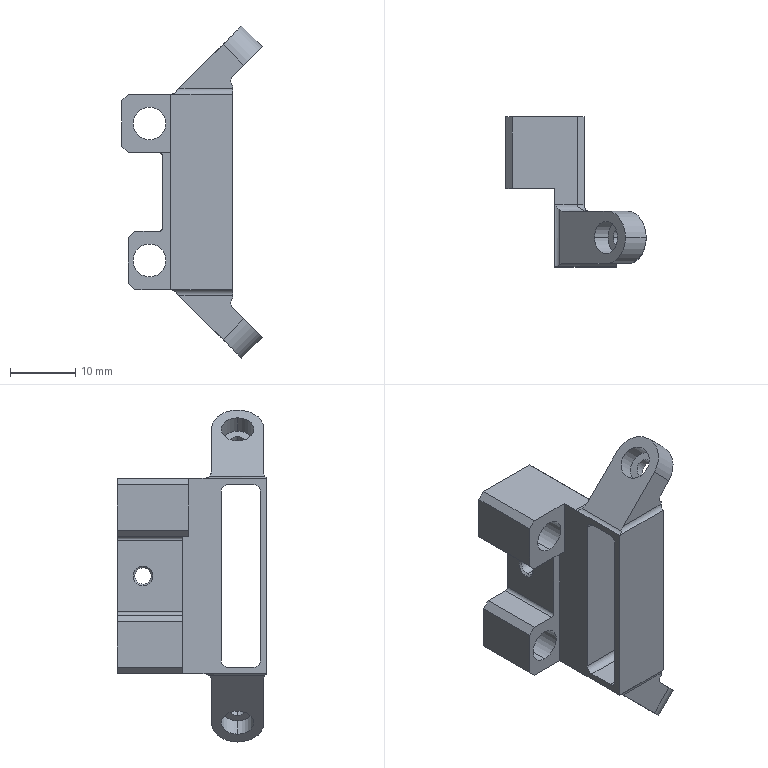NC program | NX | posted with a generic post | part box 21.534 x 23 x 50.912 mm
Lines 6134 to 6474 of 6474:
(PLANAR_MILL_1 , TOOL : D6R1)
N12248 T02 M6
N12250 G54
N12252 G17 G0 G90 X-0.5 Y-15.853 B0. C0. S1061 M3
N12254 G43 Z50. H2
N12256 Z-12.5
N12258 G94 G1 Z-14.5 F250.
N12260 X0.293 Y-13.646
N12262 X-0.414 Y-14.353
N12264 X-1.414 Y-15.353
N12266 G2 X-7. Y-17.667 R7.9
N12268 G1 X-14.
N12270 G2 X-19.586 Y-15.353 R7.9
N12272 G1 X-20.586 Y-14.353
N12274 G2 X-22.9 Y-8.767 R7.9
N12276 G1 Y0.233
N12278 G2 X-20.586 Y5.819 R7.9
N12280 G1 X-19.586 Y6.819
N12282 G2 X-14. Y9.133 R7.9
N12284 G1 X14.
N12286 G2 X19.586 Y6.819 R7.9
N12288 G1 X20.586 Y5.819
N12290 G2 X22.9 Y0.233 R7.9
N12292 G1 Y-9.767
N12294 G2 X20.586 Y-15.353 R7.9
N12296 G1 X19.586 Y-16.353
N12298 G2 X14. Y-18.667 R7.9
N12300 G1 X7.
N12302 G2 X1.414 Y-16.353 R7.9
N12304 G1 X0.414 Y-15.353
N12306 X-0.293 Y-14.646
N12308 X-0.5 Y-15.853
N12310 Z-12.5
N12312 G0 Z50.
N12314 X0.5 Y-9.61
N12316 Z-12.5
N12318 G1 Z-14.5
N12320 X-1.404 Y-11.949
N12322 X-2.111 Y-12.656
N12324 X-3.111 Y-13.656
N12326 G2 X-7. Y-15.267 R5.5
N12328 G1 X-14.
N12330 G2 X-17.889 Y-13.656 R5.5
N12332 G1 X-18.889 Y-12.656
N12334 G2 X-20.5 Y-8.767 R5.5
N12336 G1 Y0.233
N12338 G2 X-18.889 Y4.122 R5.5
N12340 G1 X-17.889 Y5.122
N12342 G2 X-14. Y6.733 R5.5
N12344 G1 X14.
N12346 G2 X17.889 Y5.122 R5.5
N12348 G1 X18.889 Y4.122
N12350 G2 X20.5 Y0.233 R5.5
N12352 G1 Y-9.767
N12354 G2 X18.889 Y-13.656 R5.5
N12356 G1 X17.889 Y-14.656
N12358 G2 X14. Y-16.267 R5.5
N12360 G1 X7.
N12362 G2 X3.111 Y-14.656 R5.5
N12364 G1 X2.111 Y-13.656
N12366 X1.404 Y-12.949
N12368 X0.5 Y-9.61
N12370 Z-12.5
N12372 G0 Z50.
N12374 X-0.98 Y-8.13
N12376 Z-12.5
N12378 G1 Z-14.5
N12380 X-3.808 Y-10.959
N12382 X-4.808 Y-11.959
N12384 G2 X-7. Y-12.867 R3.1
N12386 G1 X-14.
N12388 G2 X-16.192 Y-11.959 R3.1
N12390 G1 X-17.192 Y-10.959
N12392 G2 X-18.1 Y-8.767 R3.1
N12394 G1 Y0.233
N12396 G2 X-17.192 Y2.425 R3.1
N12398 G1 X-16.192 Y3.425
N12400 G2 X-14. Y4.333 R3.1
N12402 G1 X14.
N12404 G2 X16.192 Y3.425 R3.1
N12406 G1 X17.192 Y2.425
N12408 G2 X18.1 Y0.233 R3.1
N12410 G1 Y-9.767
N12412 G2 X17.192 Y-11.959 R3.1
N12414 G1 X16.192 Y-12.959
N12416 G2 X14. Y-13.867 R3.1
N12418 G1 X7.
N12420 G2 X4.808 Y-12.959 R3.1
N12422 G1 X3.808 Y-11.959
N12424 X0.98 Y-9.13
N12426 Z-12.5
N12428 G0 Z50.
(PLANAR_MILL_1_COPY , TOOL : D6R1)
N12430 X-1.05 Y-8.06
N12432 Z-12.5
N12434 G1 Z-14.5
N12436 X-3.879 Y-10.888
N12438 X-4.879 Y-11.888
N12440 G2 X-7. Y-12.767 R3.
N12442 G1 X-14.
N12444 G2 X-16.121 Y-11.888 R3.
N12446 G1 X-17.121 Y-10.888
N12448 G2 X-18. Y-8.767 R3.
N12450 G1 Y0.233
N12452 G2 X-17.121 Y2.354 R3.
N12454 G1 X-16.121 Y3.354
N12456 G2 X-14. Y4.233 R3.
N12458 G1 X14.
N12460 G2 X16.121 Y3.354 R3.
N12462 G1 X17.121 Y2.354
N12464 G2 X18. Y0.233 R3.
N12466 G1 Y-9.767
N12468 G2 X17.121 Y-11.888 R3.
N12470 G1 X16.121 Y-12.888
N12472 G2 X14. Y-13.767 R3.
N12474 G1 X7.
N12476 G2 X4.879 Y-12.888 R3.
N12478 G1 X3.879 Y-11.888
N12480 X1.05 Y-9.06
N12482 Z-12.5
N12484 G0 Z50.
(FLOOR_FACING_1_COPY , TOOL : D6R1)
N12486 G19 G43 Y62.5 Z-8.5 B-180. C0. H2
N12488 X0.
N12490 Y9.233
N12492 G1 Y6.233
N12494 Z-18.8
N12496 X-12.04
N12498 Z-18.7
N12500 X12.04
N12502 Z-18.8
N12504 X0.
N12506 Z-21.5
N12508 X-14.134
N12510 X-14.423 Z-21.
N12512 X-14.74
N12514 Z-16.
N12516 X14.74
N12518 Z-21.
N12520 X14.423
N12522 X14.134 Z-21.5
N12524 X0.
N12526 X-1.
N12528 Z-29.
N12530 Y9.233
N12532 G0 Y62.5
(FLOOR_FACING_1_COPY_COPY_COPY , TOOL : D6R1)
N12534 G43 Y62.5 Z6. B-180. C-180. H2
N12536 X0.
N12538 Y7.517
N12540 G1 Y4.517
N12542 Z-1.5
N12544 X2.5
N12546 Z-3.5
N12548 X0. Z-5.
N12550 X2.5 Z-3.5
N12552 Z-8.5
N12554 X-2.5
N12556 Z-1.5
N12558 X0.
N12560 X1.
N12562 Z6.
N12564 Y7.517
N12566 G0 Y62.5
(PLANAR_MILL_2 , TOOL : D6R1)
N12568 Y60.767 Z-15.
N12570 X-3.
N12572 Y6.517
N12574 G1 Y4.517
N12576 Z-11.
N12578 Z0.
N12580 Z4.
N12582 Y6.517
N12584 G0 Y60.767
N12586 X3.
N12588 Y6.517
N12590 G1 Y4.517
N12592 Z0.
N12594 Z-10.
N12596 Z-14.
N12598 Y6.517
N12600 G0 Y60.767
N12602 M5
(FLOOR_FACING_1_COPY_COPY_COPY_COPY , TOOL : D3开粗)
N12604 T03 M6
N12606 G54
N12608 G19 G0 G90 Y62.55 Z-22.3 B-180. C-180. S1061 M3
N12610 G43 X-19.55 H3
N12612 Y6.267
N12614 G94 G1 Y3.267 F250.
N12616 X-16.55
N12618 X16.55
N12620 Z-20.15
N12622 X-16.55
N12624 Z-18.
N12626 X16.55
N12628 Z-15.85
N12630 X-16.55
N12632 Z-13.7
N12634 X16.55
N12636 Z-13.5
N12638 Z-11.55
N12640 X-4.45
N12642 Y6.267
N12644 G0 Y62.55
(PLANAR_MILL_3 , TOOL : D3开粗)
N12646 Y59.767 Z-12.5
N12648 X-18.
N12650 Y6.267
N12652 G1 Y3.267
N12654 X-15.
N12656 X-6.
N12658 G18 G2 X-4.586 Y3.267 Z-11.5 R1.5
N12660 G19 G1 X15.
N12662 X18.
N12664 Y6.267
N12666 G0 Y59.767
(PLANAR_MILL , TOOL : D3开粗)
N12668 G43 Y56.233 Z-20.5 B-180. C0. H3
N12670 X1.769
N12672 Y7.233
N12674 G1 X-12.5 Y7.109
N12676 Y7.082 Z-17.5
N12678 X12.5 Y6.864
N12680 Y6.838 Z-20.5
N12682 X-12.5 Y6.62
N12684 Y6.594 Z-17.5
N12686 X12.5 Y6.376
N12688 Y6.349 Z-20.5
N12690 X-12.5 Y6.131
N12692 Y6.105 Z-17.5
N12694 X12.5 Y5.887
N12696 Y5.861 Z-20.5
N12698 X-12.5 Y5.642
N12700 Y5.616 Z-17.5
N12702 X12.5 Y5.398
N12704 Y5.372 Z-20.5
N12706 X-12.5 Y5.154
N12708 Y5.128 Z-17.5
N12710 X12.5 Y4.909
N12712 Y4.883 Z-20.5
N12714 X-12.5 Y4.665
N12716 Y4.639 Z-17.5
N12718 X12.5 Y4.421
N12720 Y4.395 Z-20.5
N12722 X-12.5 Y4.176
N12724 Y4.15 Z-17.5
N12726 X12.5 Y3.932
N12728 Y3.906 Z-20.5
N12730 X-12.5 Y3.688
N12732 Y3.661 Z-17.5
N12734 X12.5 Y3.443
N12736 Y3.417 Z-20.5
N12738 X-12.5 Y3.199
N12740 Y3.173 Z-17.5
N12742 X12.5 Y2.955
N12744 Y2.928 Z-20.5
N12746 X-12.5 Y2.71
N12748 Y2.684 Z-17.5
N12750 X12.5 Y2.466
N12752 Y2.44 Z-20.5
N12754 X-12.5 Y2.222
N12756 Y2.195 Z-17.5
N12758 X12.5 Y1.977
N12760 Y1.951 Z-20.5
N12762 X-12.5 Y1.733
N12764 Y1.707 Z-17.5
N12766 X12.5 Y1.488
N12768 Y1.462 Z-20.5
N12770 X-12.5 Y1.244
N12772 Y1.218 Z-17.5
N12774 X12.5 Y1.
N12776 Y0.974 Z-20.5
N12778 X-12.5 Y0.755
N12780 Y0.729 Z-17.5
N12782 X12.5 Y0.511
N12784 Y0.485 Z-20.5
N12786 X-12.5 Y0.267
N12788 Y0.241 Z-17.5
N12790 X12.5 Y0.022
N12792 Y-0.004 Z-20.5
N12794 X-12.5 Y-0.222
N12796 Y-0.248 Z-17.5
N12798 X12.5 Y-0.466
N12800 Y-0.493 Z-20.5
N12802 X-12.5 Y-0.711
N12804 Y-0.737 Z-17.5
N12806 X12.5 Y-0.955
N12808 Y-0.981 Z-20.5
N12810 X-12.5 Y-1.199
N12812 Y-1.226 Z-17.5
N12814 X12.5 Y-1.444
N12816 Y-1.47 Z-20.5
N12818 X-12.5 Y-1.688
N12820 Y-1.714 Z-17.5
N12822 X12.5 Y-1.932
N12824 Y-1.959 Z-20.5
N12826 X-12.5 Y-2.177
N12828 Y-2.203 Z-17.5
N12830 X12.5 Y-2.421
N12832 Y-2.447 Z-20.5
N12834 X-12.5 Y-2.665
N12836 Y-2.692 Z-17.5
N12838 X12.5 Y-2.91
N12840 Y-2.936 Z-20.5
N12842 X-12.5 Y-3.154
N12844 Y-3.18 Z-17.5
N12846 X12.5 Y-3.399
N12848 Y-3.425 Z-20.5
N12850 X-12.5 Y-3.643
N12852 Y-3.669 Z-17.5
N12854 X12.5 Y-3.887
N12856 Y-3.913 Z-20.5
N12858 X-12.5 Y-4.132
N12860 Y-4.158 Z-17.5
N12862 X0. Y-4.267
N12864 X12.5
N12866 Z-20.5
N12868 X-12.5
N12870 Z-17.5
N12872 X0.
N12874 Y-3.267
N12876 G0 Y56.233
N12878 M5
N12880 M2